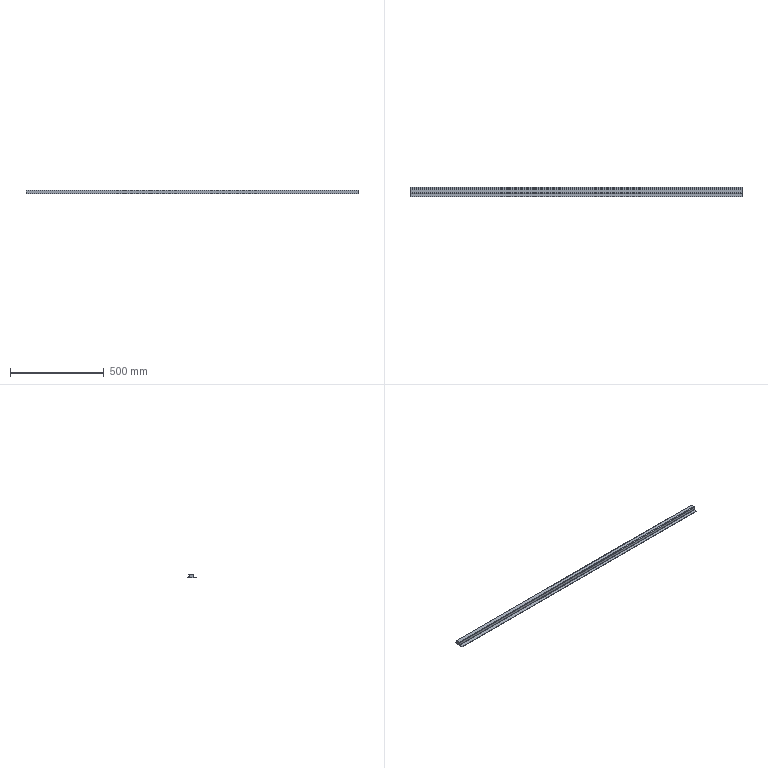Part | SolidWorks | features BaseBody 3 | 3 solids | 54 faces | box 1772 x 51 x 20 mm | volume 297636 mm3 | plane 42 | cylinder 12 | commonest cylinder face diameters 2 x8 6 x4
STEP:
#1=CARTESIAN_POINT('',(-885.9,20.5,-18.));
#2=VERTEX_POINT('',#1);
#3=CARTESIAN_POINT('',(885.9,20.5,-18.));
#4=VERTEX_POINT('',#3);
#5=CARTESIAN_POINT('',(885.9,20.5,-18.));
#6=DIRECTION('',(1.,0.,0.));
#7=VECTOR('',#6,1000.);
#8=LINE('',#5,#7);
#9=EDGE_CURVE('',#2,#4,#8,.T.);
#10=ORIENTED_EDGE('',*,*,#9,.T.);
#11=CARTESIAN_POINT('',(885.9,20.5,-20.));
#12=VERTEX_POINT('',#11);
#13=CARTESIAN_POINT('',(885.9,20.5,-20.));
#14=DIRECTION('',(0.,0.,1.));
#15=VECTOR('',#14,1000.);
#16=LINE('',#13,#15);
#17=EDGE_CURVE('',#12,#4,#16,.T.);
#18=ORIENTED_EDGE('',*,*,#17,.F.);
#19=CARTESIAN_POINT('',(-885.9,20.5,-20.));
#20=VERTEX_POINT('',#19);
#21=CARTESIAN_POINT('',(0.,20.5,-20.));
#22=DIRECTION('',(1.,0.,0.));
#23=VECTOR('',#22,1000.);
#24=LINE('',#21,#23);
#25=EDGE_CURVE('',#20,#12,#24,.T.);
#26=ORIENTED_EDGE('',*,*,#25,.F.);
#27=CARTESIAN_POINT('',(-885.9,20.5,-20.));
#28=DIRECTION('',(0.,0.,1.));
#29=VECTOR('',#28,1000.);
#30=LINE('',#27,#29);
#31=EDGE_CURVE('',#20,#2,#30,.T.);
#32=ORIENTED_EDGE('',*,*,#31,.T.);
#33=EDGE_LOOP('',(#10,#18,#26,#32));
#34=FACE_OUTER_BOUND('',#33,.T.);
#35=CARTESIAN_POINT('',(885.9,20.5,-20.));
#36=DIRECTION('',(0.,-1.,0.));
#37=DIRECTION('',(-1.,0.,0.));
#38=AXIS2_PLACEMENT_3D('',#35,#36,#37);
#39=PLANE('',#38);
#40=ADVANCED_FACE('',(#34),#39,.F.);
#41=CARTESIAN_POINT('',(-885.9,13.5,-18.));
#42=VERTEX_POINT('',#41);
#43=CARTESIAN_POINT('',(-885.9,20.5,-18.));
#44=DIRECTION('',(0.,1.,0.));
#45=VECTOR('',#44,1000.);
#46=LINE('',#43,#45);
#47=EDGE_CURVE('',#42,#2,#46,.T.);
#48=ORIENTED_EDGE('',*,*,#47,.F.);
#49=CARTESIAN_POINT('',(885.9,13.5,-18.));
#50=VERTEX_POINT('',#49);
#51=CARTESIAN_POINT('',(885.9,13.5,-18.));
#52=DIRECTION('',(-1.,0.,0.));
#53=VECTOR('',#52,1000.);
#54=LINE('',#51,#53);
#55=EDGE_CURVE('',#50,#42,#54,.T.);
#56=ORIENTED_EDGE('',*,*,#55,.F.);
#57=CARTESIAN_POINT('',(885.9,12.5,-18.));
#58=DIRECTION('',(0.,-1.,0.));
#59=VECTOR('',#58,1000.);
#60=LINE('',#57,#59);
#61=EDGE_CURVE('',#4,#50,#60,.T.);
#62=ORIENTED_EDGE('',*,*,#61,.F.);
#63=ORIENTED_EDGE('',*,*,#9,.F.);
#64=EDGE_LOOP('',(#48,#56,#62,#63));
#65=FACE_OUTER_BOUND('',#64,.T.);
#66=CARTESIAN_POINT('',(0.,0.,-18.));
#67=DIRECTION('',(0.,0.,1.));
#68=DIRECTION('',(1.,0.,0.));
#69=AXIS2_PLACEMENT_3D('',#66,#67,#68);
#70=PLANE('',#69);
#71=ADVANCED_FACE('',(#65),#70,.T.);
#72=CARTESIAN_POINT('',(-885.9,13.5,-20.));
#73=VERTEX_POINT('',#72);
#74=CARTESIAN_POINT('',(885.9,13.5,-20.));
#75=VERTEX_POINT('',#74);
#76=CARTESIAN_POINT('',(885.9,13.5,-20.));
#77=DIRECTION('',(1.,0.,0.));
#78=VECTOR('',#77,1000.);
#79=LINE('',#76,#78);
#80=EDGE_CURVE('',#73,#75,#79,.T.);
#81=ORIENTED_EDGE('',*,*,#80,.F.);
#82=CARTESIAN_POINT('',(-885.9,0.,-20.));
#83=DIRECTION('',(0.,1.,0.));
#84=VECTOR('',#83,1000.);
#85=LINE('',#82,#84);
#86=EDGE_CURVE('',#73,#20,#85,.T.);
#87=ORIENTED_EDGE('',*,*,#86,.T.);
#88=ORIENTED_EDGE('',*,*,#25,.T.);
#89=CARTESIAN_POINT('',(885.9,0.,-20.));
#90=DIRECTION('',(0.,-1.,0.));
#91=VECTOR('',#90,1000.);
#92=LINE('',#89,#91);
#93=EDGE_CURVE('',#12,#75,#92,.T.);
#94=ORIENTED_EDGE('',*,*,#93,.T.);
#95=EDGE_LOOP('',(#81,#87,#88,#94));
#96=FACE_OUTER_BOUND('',#95,.T.);
#97=CARTESIAN_POINT('',(0.,0.,-20.));
#98=DIRECTION('',(0.,0.,1.));
#99=DIRECTION('',(1.,0.,0.));
#100=AXIS2_PLACEMENT_3D('',#97,#98,#99);
#101=PLANE('',#100);
#102=ADVANCED_FACE('',(#96),#101,.F.);
#103=CARTESIAN_POINT('',(885.9,13.5,-20.));
#104=DIRECTION('',(0.,0.,-1.));
#105=VECTOR('',#104,1000.);
#106=LINE('',#103,#105);
#107=EDGE_CURVE('',#50,#75,#106,.T.);
#108=ORIENTED_EDGE('',*,*,#107,.T.);
#109=ORIENTED_EDGE('',*,*,#93,.F.);
#110=ORIENTED_EDGE('',*,*,#17,.T.);
#111=ORIENTED_EDGE('',*,*,#61,.T.);
#112=EDGE_LOOP('',(#108,#109,#110,#111));
#113=FACE_OUTER_BOUND('',#112,.T.);
#114=CARTESIAN_POINT('',(885.9,12.5,-20.));
#115=DIRECTION('',(-1.,0.,0.));
#116=DIRECTION('',(0.,0.,1.));
#117=AXIS2_PLACEMENT_3D('',#114,#115,#116);
#118=PLANE('',#117);
#119=ADVANCED_FACE('',(#113),#118,.F.);
#120=CARTESIAN_POINT('',(-885.9,13.5,-18.));
#121=DIRECTION('',(0.,0.,-1.));
#122=VECTOR('',#121,1000.);
#123=LINE('',#120,#122);
#124=EDGE_CURVE('',#42,#73,#123,.T.);
#125=ORIENTED_EDGE('',*,*,#124,.F.);
#126=ORIENTED_EDGE('',*,*,#47,.T.);
#127=ORIENTED_EDGE('',*,*,#31,.F.);
#128=ORIENTED_EDGE('',*,*,#86,.F.);
#129=EDGE_LOOP('',(#125,#126,#127,#128));
#130=FACE_OUTER_BOUND('',#129,.T.);
#131=CARTESIAN_POINT('',(-885.9,20.5,-20.));
#132=DIRECTION('',(1.,0.,0.));
#133=DIRECTION('',(0.,1.,0.));
#134=AXIS2_PLACEMENT_3D('',#131,#132,#133);
#135=PLANE('',#134);
#136=ADVANCED_FACE('',(#130),#135,.F.);
#137=CARTESIAN_POINT('',(-885.9,12.5,-17.));
#138=VERTEX_POINT('',#137);
#139=CARTESIAN_POINT('',(885.9,12.5,-17.));
#140=VERTEX_POINT('',#139);
#141=CARTESIAN_POINT('',(-885.9,12.5,-17.));
#142=DIRECTION('',(1.,0.,0.));
#143=VECTOR('',#142,1000.);
#144=LINE('',#141,#143);
#145=EDGE_CURVE('',#138,#140,#144,.T.);
#146=ORIENTED_EDGE('',*,*,#145,.T.);
#147=CARTESIAN_POINT('',(885.9,13.5,-17.));
#148=DIRECTION('',(1.,0.,0.));
#149=DIRECTION('',(0.,0.,1.));
#150=AXIS2_PLACEMENT_3D('',#147,#148,#149);
#151=CIRCLE('',#150,1.);
#152=EDGE_CURVE('',#140,#50,#151,.T.);
#153=ORIENTED_EDGE('',*,*,#152,.T.);
#154=ORIENTED_EDGE('',*,*,#55,.T.);
#155=CARTESIAN_POINT('',(-885.9,13.5,-17.));
#156=DIRECTION('',(-1.,0.,0.));
#157=DIRECTION('',(0.,0.,1.));
#158=AXIS2_PLACEMENT_3D('',#155,#156,#157);
#159=CIRCLE('',#158,1.);
#160=EDGE_CURVE('',#42,#138,#159,.T.);
#161=ORIENTED_EDGE('',*,*,#160,.T.);
#162=EDGE_LOOP('',(#146,#153,#154,#161));
#163=FACE_OUTER_BOUND('',#162,.T.);
#164=CARTESIAN_POINT('',(-885.9,13.5,-17.));
#165=DIRECTION('',(-1.,0.,0.));
#166=DIRECTION('',(0.,0.,-1.));
#167=AXIS2_PLACEMENT_3D('',#164,#165,#166);
#168=CYLINDRICAL_SURFACE('',#167,1.);
#169=ADVANCED_FACE('',(#163),#168,.F.);
#170=CARTESIAN_POINT('',(-885.9,10.5,-17.));
#171=VERTEX_POINT('',#170);
#172=CARTESIAN_POINT('',(885.9,10.5,-17.));
#173=VERTEX_POINT('',#172);
#174=CARTESIAN_POINT('',(-885.9,10.5,-17.));
#175=DIRECTION('',(1.,0.,0.));
#176=VECTOR('',#175,1000.);
#177=LINE('',#174,#176);
#178=EDGE_CURVE('',#171,#173,#177,.T.);
#179=ORIENTED_EDGE('',*,*,#178,.F.);
#180=CARTESIAN_POINT('',(-885.9,13.5,-17.));
#181=DIRECTION('',(-1.,0.,0.));
#182=DIRECTION('',(0.,0.,1.));
#183=AXIS2_PLACEMENT_3D('',#180,#181,#182);
#184=CIRCLE('',#183,3.);
#185=EDGE_CURVE('',#73,#171,#184,.T.);
#186=ORIENTED_EDGE('',*,*,#185,.F.);
#187=ORIENTED_EDGE('',*,*,#80,.T.);
#188=CARTESIAN_POINT('',(885.9,13.5,-17.));
#189=DIRECTION('',(1.,0.,0.));
#190=DIRECTION('',(0.,0.,1.));
#191=AXIS2_PLACEMENT_3D('',#188,#189,#190);
#192=CIRCLE('',#191,3.);
#193=EDGE_CURVE('',#173,#75,#192,.T.);
#194=ORIENTED_EDGE('',*,*,#193,.F.);
#195=EDGE_LOOP('',(#179,#186,#187,#194));
#196=FACE_OUTER_BOUND('',#195,.T.);
#197=CARTESIAN_POINT('',(-885.9,13.5,-17.));
#198=DIRECTION('',(-1.,0.,0.));
#199=DIRECTION('',(0.,0.,-1.));
#200=AXIS2_PLACEMENT_3D('',#197,#198,#199);
#201=CYLINDRICAL_SURFACE('',#200,3.);
#202=ADVANCED_FACE('',(#196),#201,.T.);
#203=ORIENTED_EDGE('',*,*,#160,.F.);
#204=ORIENTED_EDGE('',*,*,#124,.T.);
#205=ORIENTED_EDGE('',*,*,#185,.T.);
#206=CARTESIAN_POINT('',(-885.9,12.5,-17.));
#207=DIRECTION('',(0.,-1.,0.));
#208=VECTOR('',#207,1000.);
#209=LINE('',#206,#208);
#210=EDGE_CURVE('',#138,#171,#209,.T.);
#211=ORIENTED_EDGE('',*,*,#210,.F.);
#212=EDGE_LOOP('',(#203,#204,#205,#211));
#213=FACE_OUTER_BOUND('',#212,.T.);
#214=CARTESIAN_POINT('',(-885.9,13.5,-17.));
#215=DIRECTION('',(1.,0.,0.));
#216=DIRECTION('',(0.,1.,0.));
#217=AXIS2_PLACEMENT_3D('',#214,#215,#216);
#218=PLANE('',#217);
#219=ADVANCED_FACE('',(#213),#218,.F.);
#220=ORIENTED_EDGE('',*,*,#107,.F.);
#221=ORIENTED_EDGE('',*,*,#152,.F.);
#222=CARTESIAN_POINT('',(885.9,12.5,-17.));
#223=DIRECTION('',(0.,-1.,0.));
#224=VECTOR('',#223,1000.);
#225=LINE('',#222,#224);
#226=EDGE_CURVE('',#140,#173,#225,.T.);
#227=ORIENTED_EDGE('',*,*,#226,.T.);
#228=ORIENTED_EDGE('',*,*,#193,.T.);
#229=EDGE_LOOP('',(#220,#221,#227,#228));
#230=FACE_OUTER_BOUND('',#229,.T.);
#231=CARTESIAN_POINT('',(885.9,13.5,-17.));
#232=DIRECTION('',(1.,0.,0.));
#233=DIRECTION('',(0.,1.,0.));
#234=AXIS2_PLACEMENT_3D('',#231,#232,#233);
#235=PLANE('',#234);
#236=ADVANCED_FACE('',(#230),#235,.T.);
#237=CARTESIAN_POINT('',(-885.9,-30.5,-18.));
#238=VERTEX_POINT('',#237);
#239=CARTESIAN_POINT('',(885.9,-30.5,-18.));
#240=VERTEX_POINT('',#239);
#241=CARTESIAN_POINT('',(0.,-30.5,-18.));
#242=DIRECTION('',(1.,0.,0.));
#243=VECTOR('',#242,1000.);
#244=LINE('',#241,#243);
#245=EDGE_CURVE('',#238,#240,#244,.T.);
#246=ORIENTED_EDGE('',*,*,#245,.F.);
#247=CARTESIAN_POINT('',(-885.9,-30.5,-20.));
#248=VERTEX_POINT('',#247);
#249=CARTESIAN_POINT('',(-885.9,-30.5,-20.));
#250=DIRECTION('',(0.,0.,1.));
#251=VECTOR('',#250,1000.);
#252=LINE('',#249,#251);
#253=EDGE_CURVE('',#248,#238,#252,.T.);
#254=ORIENTED_EDGE('',*,*,#253,.F.);
#255=CARTESIAN_POINT('',(885.9,-30.5,-20.));
#256=VERTEX_POINT('',#255);
#257=CARTESIAN_POINT('',(-885.9,-30.5,-20.));
#258=DIRECTION('',(1.,0.,0.));
#259=VECTOR('',#258,1000.);
#260=LINE('',#257,#259);
#261=EDGE_CURVE('',#248,#256,#260,.T.);
#262=ORIENTED_EDGE('',*,*,#261,.T.);
#263=CARTESIAN_POINT('',(885.9,-30.5,-20.));
#264=DIRECTION('',(0.,0.,1.));
#265=VECTOR('',#264,1000.);
#266=LINE('',#263,#265);
#267=EDGE_CURVE('',#256,#240,#266,.T.);
#268=ORIENTED_EDGE('',*,*,#267,.T.);
#269=EDGE_LOOP('',(#246,#254,#262,#268));
#270=FACE_OUTER_BOUND('',#269,.T.);
#271=CARTESIAN_POINT('',(-885.9,-30.5,-20.));
#272=DIRECTION('',(0.,-1.,0.));
#273=DIRECTION('',(0.,0.,-1.));
#274=AXIS2_PLACEMENT_3D('',#271,#272,#273);
#275=PLANE('',#274);
#276=ADVANCED_FACE('',(#270),#275,.T.);
#277=CARTESIAN_POINT('',(885.9,-13.5,-18.));
#278=VERTEX_POINT('',#277);
#279=CARTESIAN_POINT('',(885.9,0.,-18.));
#280=DIRECTION('',(0.,1.,0.));
#281=VECTOR('',#280,1000.);
#282=LINE('',#279,#281);
#283=EDGE_CURVE('',#240,#278,#282,.T.);
#284=ORIENTED_EDGE('',*,*,#283,.T.);
#285=CARTESIAN_POINT('',(-885.9,-13.5,-18.));
#286=VERTEX_POINT('',#285);
#287=CARTESIAN_POINT('',(-885.9,-13.5,-18.));
#288=DIRECTION('',(1.,0.,0.));
#289=VECTOR('',#288,1000.);
#290=LINE('',#287,#289);
#291=EDGE_CURVE('',#286,#278,#290,.T.);
#292=ORIENTED_EDGE('',*,*,#291,.F.);
#293=CARTESIAN_POINT('',(-885.9,0.,-18.));
#294=DIRECTION('',(0.,-1.,0.));
#295=VECTOR('',#294,1000.);
#296=LINE('',#293,#295);
#297=EDGE_CURVE('',#286,#238,#296,.T.);
#298=ORIENTED_EDGE('',*,*,#297,.T.);
#299=ORIENTED_EDGE('',*,*,#245,.T.);
#300=EDGE_LOOP('',(#284,#292,#298,#299));
#301=FACE_OUTER_BOUND('',#300,.T.);
#302=CARTESIAN_POINT('',(0.,0.,-18.));
#303=DIRECTION('',(0.,0.,1.));
#304=DIRECTION('',(1.,0.,0.));
#305=AXIS2_PLACEMENT_3D('',#302,#303,#304);
#306=PLANE('',#305);
#307=ADVANCED_FACE('',(#301),#306,.T.);
#308=CARTESIAN_POINT('',(885.9,-13.5,-20.));
#309=VERTEX_POINT('',#308);
#310=CARTESIAN_POINT('',(-885.9,-13.5,-20.));
#311=VERTEX_POINT('',#310);
#312=CARTESIAN_POINT('',(-885.9,-13.5,-20.));
#313=DIRECTION('',(-1.,0.,0.));
#314=VECTOR('',#313,1000.);
#315=LINE('',#312,#314);
#316=EDGE_CURVE('',#309,#311,#315,.T.);
#317=ORIENTED_EDGE('',*,*,#316,.F.);
#318=CARTESIAN_POINT('',(885.9,-30.5,-20.));
#319=DIRECTION('',(0.,1.,0.));
#320=VECTOR('',#319,1000.);
#321=LINE('',#318,#320);
#322=EDGE_CURVE('',#256,#309,#321,.T.);
#323=ORIENTED_EDGE('',*,*,#322,.F.);
#324=ORIENTED_EDGE('',*,*,#261,.F.);
#325=CARTESIAN_POINT('',(-885.9,-12.5,-20.));
#326=DIRECTION('',(0.,-1.,0.));
#327=VECTOR('',#326,1000.);
#328=LINE('',#325,#327);
#329=EDGE_CURVE('',#311,#248,#328,.T.);
#330=ORIENTED_EDGE('',*,*,#329,.F.);
#331=EDGE_LOOP('',(#317,#323,#324,#330));
#332=FACE_OUTER_BOUND('',#331,.T.);
#333=CARTESIAN_POINT('',(0.,0.,-20.));
#334=DIRECTION('',(0.,0.,1.));
#335=DIRECTION('',(1.,0.,0.));
#336=AXIS2_PLACEMENT_3D('',#333,#334,#335);
#337=PLANE('',#336);
#338=ADVANCED_FACE('',(#332),#337,.F.);
#339=ORIENTED_EDGE('',*,*,#322,.T.);
#340=CARTESIAN_POINT('',(885.9,-13.5,-18.));
#341=DIRECTION('',(0.,0.,-1.));
#342=VECTOR('',#341,1000.);
#343=LINE('',#340,#342);
#344=EDGE_CURVE('',#278,#309,#343,.T.);
#345=ORIENTED_EDGE('',*,*,#344,.F.);
#346=ORIENTED_EDGE('',*,*,#283,.F.);
#347=ORIENTED_EDGE('',*,*,#267,.F.);
#348=EDGE_LOOP('',(#339,#345,#346,#347));
#349=FACE_OUTER_BOUND('',#348,.T.);
#350=CARTESIAN_POINT('',(885.9,-30.5,-20.));
#351=DIRECTION('',(1.,0.,0.));
#352=DIRECTION('',(0.,0.,-1.));
#353=AXIS2_PLACEMENT_3D('',#350,#351,#352);
#354=PLANE('',#353);
#355=ADVANCED_FACE('',(#349),#354,.T.);
#356=ORIENTED_EDGE('',*,*,#297,.F.);
#357=CARTESIAN_POINT('',(-885.9,-13.5,-20.));
#358=DIRECTION('',(0.,0.,-1.));
#359=VECTOR('',#358,1000.);
#360=LINE('',#357,#359);
#361=EDGE_CURVE('',#286,#311,#360,.T.);
#362=ORIENTED_EDGE('',*,*,#361,.T.);
#363=ORIENTED_EDGE('',*,*,#329,.T.);
#364=ORIENTED_EDGE('',*,*,#253,.T.);
#365=EDGE_LOOP('',(#356,#362,#363,#364));
#366=FACE_OUTER_BOUND('',#365,.T.);
#367=CARTESIAN_POINT('',(-885.9,-12.5,-20.));
#368=DIRECTION('',(-1.,0.,0.));
#369=DIRECTION('',(0.,1.,0.));
#370=AXIS2_PLACEMENT_3D('',#367,#368,#369);
#371=PLANE('',#370);
#372=ADVANCED_FACE('',(#366),#371,.T.);
#373=CARTESIAN_POINT('',(885.9,-12.5,-17.));
#374=VERTEX_POINT('',#373);
#375=CARTESIAN_POINT('',(-885.9,-12.5,-17.));
#376=VERTEX_POINT('',#375);
#377=CARTESIAN_POINT('',(885.9,-12.5,-17.));
#378=DIRECTION('',(-1.,0.,0.));
#379=VECTOR('',#378,1000.);
#380=LINE('',#377,#379);
#381=EDGE_CURVE('',#374,#376,#380,.T.);
#382=ORIENTED_EDGE('',*,*,#381,.T.);
#383=CARTESIAN_POINT('',(-885.9,-13.5,-17.));
#384=DIRECTION('',(-1.,0.,0.));
#385=DIRECTION('',(0.,0.,-1.));
#386=AXIS2_PLACEMENT_3D('',#383,#384,#385);
#387=CIRCLE('',#386,1.);
#388=EDGE_CURVE('',#376,#286,#387,.T.);
#389=ORIENTED_EDGE('',*,*,#388,.T.);
#390=ORIENTED_EDGE('',*,*,#291,.T.);
#391=CARTESIAN_POINT('',(885.9,-13.5,-17.));
#392=DIRECTION('',(1.,0.,0.));
#393=DIRECTION('',(0.,0.,-1.));
#394=AXIS2_PLACEMENT_3D('',#391,#392,#393);
#395=CIRCLE('',#394,1.);
#396=EDGE_CURVE('',#278,#374,#395,.T.);
#397=ORIENTED_EDGE('',*,*,#396,.T.);
#398=EDGE_LOOP('',(#382,#389,#390,#397));
#399=FACE_OUTER_BOUND('',#398,.T.);
#400=CARTESIAN_POINT('',(885.9,-13.5,-17.));
#401=DIRECTION('',(1.,0.,0.));
#402=DIRECTION('',(0.,0.,-1.));
#403=AXIS2_PLACEMENT_3D('',#400,#401,#402);
#404=CYLINDRICAL_SURFACE('',#403,1.);
#405=ADVANCED_FACE('',(#399),#404,.F.);
#406=CARTESIAN_POINT('',(885.9,-10.5,-17.));
#407=VERTEX_POINT('',#406);
#408=CARTESIAN_POINT('',(-885.9,-10.5,-17.));
#409=VERTEX_POINT('',#408);
#410=CARTESIAN_POINT('',(885.9,-10.5,-17.));
#411=DIRECTION('',(-1.,0.,0.));
#412=VECTOR('',#411,1000.);
#413=LINE('',#410,#412);
#414=EDGE_CURVE('',#407,#409,#413,.T.);
#415=ORIENTED_EDGE('',*,*,#414,.F.);
#416=CARTESIAN_POINT('',(885.9,-13.5,-17.));
#417=DIRECTION('',(1.,0.,0.));
#418=DIRECTION('',(0.,0.,-1.));
#419=AXIS2_PLACEMENT_3D('',#416,#417,#418);
#420=CIRCLE('',#419,3.);
#421=EDGE_CURVE('',#309,#407,#420,.T.);
#422=ORIENTED_EDGE('',*,*,#421,.F.);
#423=ORIENTED_EDGE('',*,*,#316,.T.);
#424=CARTESIAN_POINT('',(-885.9,-13.5,-17.));
#425=DIRECTION('',(-1.,0.,0.));
#426=DIRECTION('',(0.,0.,-1.));
#427=AXIS2_PLACEMENT_3D('',#424,#425,#426);
#428=CIRCLE('',#427,3.);
#429=EDGE_CURVE('',#409,#311,#428,.T.);
#430=ORIENTED_EDGE('',*,*,#429,.F.);
#431=EDGE_LOOP('',(#415,#422,#423,#430));
#432=FACE_OUTER_BOUND('',#431,.T.);
#433=CARTESIAN_POINT('',(885.9,-13.5,-17.));
#434=DIRECTION('',(1.,0.,0.));
#435=DIRECTION('',(0.,0.,-1.));
#436=AXIS2_PLACEMENT_3D('',#433,#434,#435);
#437=CYLINDRICAL_SURFACE('',#436,3.);
#438=ADVANCED_FACE('',(#432),#437,.T.);
#439=ORIENTED_EDGE('',*,*,#396,.F.);
#440=ORIENTED_EDGE('',*,*,#344,.T.);
#441=ORIENTED_EDGE('',*,*,#421,.T.);
#442=CARTESIAN_POINT('',(885.9,-12.5,-17.));
#443=DIRECTION('',(0.,1.,0.));
#444=VECTOR('',#443,1000.);
#445=LINE('',#442,#444);
#446=EDGE_CURVE('',#374,#407,#445,.T.);
#447=ORIENTED_EDGE('',*,*,#446,.F.);
#448=EDGE_LOOP('',(#439,#440,#441,#447));
#449=FACE_OUTER_BOUND('',#448,.T.);
#450=CARTESIAN_POINT('',(885.9,-13.5,-17.));
#451=DIRECTION('',(-1.,0.,0.));
#452=DIRECTION('',(0.,0.,1.));
#453=AXIS2_PLACEMENT_3D('',#450,#451,#452);
#454=PLANE('',#453);
#455=ADVANCED_FACE('',(#449),#454,.F.);
#456=ORIENTED_EDGE('',*,*,#361,.F.);
#457=ORIENTED_EDGE('',*,*,#388,.F.);
#458=CARTESIAN_POINT('',(-885.9,-12.5,-17.));
#459=DIRECTION('',(0.,1.,0.));
#460=VECTOR('',#459,1000.);
#461=LINE('',#458,#460);
#462=EDGE_CURVE('',#376,#409,#461,.T.);
#463=ORIENTED_EDGE('',*,*,#462,.T.);
#464=ORIENTED_EDGE('',*,*,#429,.T.);
#465=EDGE_LOOP('',(#456,#457,#463,#464));
#466=FACE_OUTER_BOUND('',#465,.T.);
#467=CARTESIAN_POINT('',(-885.9,-13.5,-17.));
#468=DIRECTION('',(-1.,0.,0.));
#469=DIRECTION('',(0.,0.,1.));
#470=AXIS2_PLACEMENT_3D('',#467,#468,#469);
#471=PLANE('',#470);
#472=ADVANCED_FACE('',(#466),#471,.T.);
#473=ORIENTED_EDGE('',*,*,#462,.F.);
#474=CARTESIAN_POINT('',(-885.9,-12.5,-3.));
#475=VERTEX_POINT('',#474);
#476=CARTESIAN_POINT('',(-885.9,-12.5,-20.));
#477=DIRECTION('',(0.,0.,1.));
#478=VECTOR('',#477,1000.);
#479=LINE('',#476,#478);
#480=EDGE_CURVE('',#376,#475,#479,.T.);
#481=ORIENTED_EDGE('',*,*,#480,.T.);
#482=CARTESIAN_POINT('',(-885.9,-10.5,-3.));
#483=VERTEX_POINT('',#482);
#484=CARTESIAN_POINT('',(-885.9,-10.5,-3.));
#485=DIRECTION('',(0.,-1.,0.));
#486=VECTOR('',#485,1000.);
#487=LINE('',#484,#486);
#488=EDGE_CURVE('',#483,#475,#487,.T.);
#489=ORIENTED_EDGE('',*,*,#488,.F.);
#490=CARTESIAN_POINT('',(-885.9,-10.5,0.));
#491=DIRECTION('',(0.,0.,1.));
#492=VECTOR('',#491,1000.);
#493=LINE('',#490,#492);
#494=EDGE_CURVE('',#409,#483,#493,.T.);
#495=ORIENTED_EDGE('',*,*,#494,.F.);
#496=EDGE_LOOP('',(#473,#481,#489,#495));
#497=FACE_OUTER_BOUND('',#496,.T.);
#498=CARTESIAN_POINT('',(-885.9,-12.5,-20.));
#499=DIRECTION('',(-1.,0.,0.));
#500=DIRECTION('',(0.,0.,1.));
#501=AXIS2_PLACEMENT_3D('',#498,#499,#500);
#502=PLANE('',#501);
#503=ADVANCED_FACE('',(#497),#502,.T.);
#504=CARTESIAN_POINT('',(-885.9,-9.5,-2.));
#505=VERTEX_POINT('',#504);
#506=CARTESIAN_POINT('',(885.9,-9.5,-2.));
#507=VERTEX_POINT('',#506);
#508=CARTESIAN_POINT('',(-885.9,-9.5,-2.));
#509=DIRECTION('',(1.,0.,0.));
#510=VECTOR('',#509,1000.);
#511=LINE('',#508,#510);
#512=EDGE_CURVE('',#505,#507,#511,.T.);
#513=ORIENTED_EDGE('',*,*,#512,.T.);
#514=CARTESIAN_POINT('',(885.9,-10.5,-3.));
#515=VERTEX_POINT('',#514);
#516=CARTESIAN_POINT('',(885.9,-9.5,-3.));
#517=DIRECTION('',(1.,0.,0.));
#518=DIRECTION('',(0.,0.,1.));
#519=AXIS2_PLACEMENT_3D('',#516,#517,#518);
#520=CIRCLE('',#519,1.);
#521=EDGE_CURVE('',#507,#515,#520,.T.);
#522=ORIENTED_EDGE('',*,*,#521,.T.);
#523=CARTESIAN_POINT('',(885.9,-10.5,-3.));
#524=DIRECTION('',(-1.,0.,0.));
#525=VECTOR('',#524,1000.);
#526=LINE('',#523,#525);
#527=EDGE_CURVE('',#515,#483,#526,.T.);
#528=ORIENTED_EDGE('',*,*,#527,.T.);
#529=CARTESIAN_POINT('',(-885.9,-9.5,-3.));
#530=DIRECTION('',(-1.,0.,0.));
#531=DIRECTION('',(0.,0.,1.));
#532=AXIS2_PLACEMENT_3D('',#529,#530,#531);
#533=CIRCLE('',#532,1.);
#534=EDGE_CURVE('',#483,#505,#533,.T.);
#535=ORIENTED_EDGE('',*,*,#534,.T.);
#536=EDGE_LOOP('',(#513,#522,#528,#535));
#537=FACE_OUTER_BOUND('',#536,.T.);
#538=CARTESIAN_POINT('',(-885.9,-9.5,-3.));
#539=DIRECTION('',(-1.,0.,0.));
#540=DIRECTION('',(0.,-1.,0.));
#541=AXIS2_PLACEMENT_3D('',#538,#539,#540);
#542=CYLINDRICAL_SURFACE('',#541,1.);
#543=ADVANCED_FACE('',(#537),#542,.F.);
#544=CARTESIAN_POINT('',(-885.9,-9.5,0.));
#545=VERTEX_POINT('',#544);
#546=CARTESIAN_POINT('',(885.9,-9.5,0.));
#547=VERTEX_POINT('',#546);
#548=CARTESIAN_POINT('',(-885.9,-9.5,0.));
#549=DIRECTION('',(1.,0.,0.));
#550=VECTOR('',#549,1000.);
#551=LINE('',#548,#550);
#552=EDGE_CURVE('',#545,#547,#551,.T.);
#553=ORIENTED_EDGE('',*,*,#552,.F.);
#554=CARTESIAN_POINT('',(-885.9,-9.5,-3.));
#555=DIRECTION('',(-1.,0.,0.));
#556=DIRECTION('',(0.,0.,1.));
#557=AXIS2_PLACEMENT_3D('',#554,#555,#556);
#558=CIRCLE('',#557,3.);
#559=EDGE_CURVE('',#475,#545,#558,.T.);
#560=ORIENTED_EDGE('',*,*,#559,.F.);
#561=CARTESIAN_POINT('',(885.9,-12.5,-3.));
#562=VERTEX_POINT('',#561);
#563=CARTESIAN_POINT('',(885.9,-12.5,-3.));
#564=DIRECTION('',(1.,0.,0.));
#565=VECTOR('',#564,1000.);
#566=LINE('',#563,#565);
#567=EDGE_CURVE('',#475,#562,#566,.T.);
#568=ORIENTED_EDGE('',*,*,#567,.T.);
#569=CARTESIAN_POINT('',(885.9,-9.5,-3.));
#570=DIRECTION('',(1.,0.,0.));
#571=DIRECTION('',(0.,0.,1.));
#572=AXIS2_PLACEMENT_3D('',#569,#570,#571);
#573=CIRCLE('',#572,3.);
#574=EDGE_CURVE('',#547,#562,#573,.T.);
#575=ORIENTED_EDGE('',*,*,#574,.F.);
#576=EDGE_LOOP('',(#553,#560,#568,#575));
#577=FACE_OUTER_BOUND('',#576,.T.);
#578=CARTESIAN_POINT('',(-885.9,-9.5,-3.));
#579=DIRECTION('',(-1.,0.,0.));
#580=DIRECTION('',(0.,-1.,0.));
#581=AXIS2_PLACEMENT_3D('',#578,#579,#580);
#582=CYLINDRICAL_SURFACE('',#581,3.);
#583=ADVANCED_FACE('',(#577),#582,.T.);
#584=ORIENTED_EDGE('',*,*,#534,.F.);
#585=ORIENTED_EDGE('',*,*,#488,.T.);
#586=ORIENTED_EDGE('',*,*,#559,.T.);
#587=CARTESIAN_POINT('',(-885.9,-9.5,-2.));
#588=DIRECTION('',(0.,0.,1.));
#589=VECTOR('',#588,1000.);
#590=LINE('',#587,#589);
#591=EDGE_CURVE('',#505,#545,#590,.T.);
#592=ORIENTED_EDGE('',*,*,#591,.F.);
#593=EDGE_LOOP('',(#584,#585,#586,#592));
#594=FACE_OUTER_BOUND('',#593,.T.);
#595=CARTESIAN_POINT('',(-885.9,-9.5,-3.));
#596=DIRECTION('',(1.,0.,0.));
#597=DIRECTION('',(0.,1.,0.));
#598=AXIS2_PLACEMENT_3D('',#595,#596,#597);
#599=PLANE('',#598);
#600=ADVANCED_FACE('',(#594),#599,.F.);
#601=CARTESIAN_POINT('',(885.9,-12.5,-3.));
#602=DIRECTION('',(0.,-1.,0.));
#603=VECTOR('',#602,1000.);
#604=LINE('',#601,#603);
#605=EDGE_CURVE('',#515,#562,#604,.T.);
#606=ORIENTED_EDGE('',*,*,#605,.F.);
#607=ORIENTED_EDGE('',*,*,#521,.F.);
#608=CARTESIAN_POINT('',(885.9,-9.5,-2.));
#609=DIRECTION('',(0.,0.,1.));
#610=VECTOR('',#609,1000.);
#611=LINE('',#608,#610);
#612=EDGE_CURVE('',#507,#547,#611,.T.);
#613=ORIENTED_EDGE('',*,*,#612,.T.);
#614=ORIENTED_EDGE('',*,*,#574,.T.);
#615=EDGE_LOOP('',(#606,#607,#613,#614));
#616=FACE_OUTER_BOUND('',#615,.T.);
#617=CARTESIAN_POINT('',(885.9,-9.5,-3.));
#618=DIRECTION('',(1.,0.,0.));
#619=DIRECTION('',(0.,1.,0.));
#620=AXIS2_PLACEMENT_3D('',#617,#618,#619);
#621=PLANE('',#620);
#622=ADVANCED_FACE('',(#616),#621,.T.);
#623=ORIENTED_EDGE('',*,*,#226,.F.);
#624=CARTESIAN_POINT('',(885.9,12.5,-3.));
#625=VERTEX_POINT('',#624);
#626=CARTESIAN_POINT('',(885.9,12.5,-2.));
#627=DIRECTION('',(0.,0.,1.));
#628=VECTOR('',#627,1000.);
#629=LINE('',#626,#628);
#630=EDGE_CURVE('',#140,#625,#629,.T.);
#631=ORIENTED_EDGE('',*,*,#630,.T.);
#632=CARTESIAN_POINT('',(885.9,10.5,-3.));
#633=VERTEX_POINT('',#632);
#634=CARTESIAN_POINT('',(885.9,10.5,-3.));
#635=DIRECTION('',(0.,1.,0.));
#636=VECTOR('',#635,1000.);
#637=LINE('',#634,#636);
#638=EDGE_CURVE('',#633,#625,#637,.T.);
#639=ORIENTED_EDGE('',*,*,#638,.F.);
#640=CARTESIAN_POINT('',(885.9,10.5,0.));
#641=DIRECTION('',(0.,0.,1.));
#642=VECTOR('',#641,1000.);
#643=LINE('',#640,#642);
#644=EDGE_CURVE('',#173,#633,#643,.T.);
#645=ORIENTED_EDGE('',*,*,#644,.F.);
#646=EDGE_LOOP('',(#623,#631,#639,#645));
#647=FACE_OUTER_BOUND('',#646,.T.);
#648=CARTESIAN_POINT('',(885.9,12.5,-2.));
#649=DIRECTION('',(1.,0.,0.));
#650=DIRECTION('',(0.,1.,0.));
#651=AXIS2_PLACEMENT_3D('',#648,#649,#650);
#652=PLANE('',#651);
#653=ADVANCED_FACE('',(#647),#652,.T.);
#654=CARTESIAN_POINT('',(885.9,9.5,-2.));
#655=VERTEX_POINT('',#654);
#656=CARTESIAN_POINT('',(-885.9,9.5,-2.));
#657=VERTEX_POINT('',#656);
#658=CARTESIAN_POINT('',(885.9,9.5,-2.));
#659=DIRECTION('',(-1.,0.,0.));
#660=VECTOR('',#659,1000.);
#661=LINE('',#658,#660);
#662=EDGE_CURVE('',#655,#657,#661,.T.);
#663=ORIENTED_EDGE('',*,*,#662,.T.);
#664=CARTESIAN_POINT('',(-885.9,10.5,-3.));
#665=VERTEX_POINT('',#664);
#666=CARTESIAN_POINT('',(-885.9,9.5,-3.));
#667=DIRECTION('',(-1.,0.,0.));
#668=DIRECTION('',(0.,0.,-1.));
#669=AXIS2_PLACEMENT_3D('',#666,#667,#668);
#670=CIRCLE('',#669,1.);
#671=EDGE_CURVE('',#657,#665,#670,.T.);
#672=ORIENTED_EDGE('',*,*,#671,.T.);
#673=CARTESIAN_POINT('',(-885.9,10.5,-3.));
#674=DIRECTION('',(1.,0.,0.));
#675=VECTOR('',#674,1000.);
#676=LINE('',#673,#675);
#677=EDGE_CURVE('',#665,#633,#676,.T.);
#678=ORIENTED_EDGE('',*,*,#677,.T.);
#679=CARTESIAN_POINT('',(885.9,9.5,-3.));
#680=DIRECTION('',(1.,0.,0.));
#681=DIRECTION('',(0.,0.,-1.));
#682=AXIS2_PLACEMENT_3D('',#679,#680,#681);
#683=CIRCLE('',#682,1.);
#684=EDGE_CURVE('',#633,#655,#683,.T.);
#685=ORIENTED_EDGE('',*,*,#684,.T.);
#686=EDGE_LOOP('',(#663,#672,#678,#685));
#687=FACE_OUTER_BOUND('',#686,.T.);
#688=CARTESIAN_POINT('',(885.9,9.5,-3.));
#689=DIRECTION('',(1.,0.,0.));
#690=DIRECTION('',(0.,1.,0.));
#691=AXIS2_PLACEMENT_3D('',#688,#689,#690);
#692=CYLINDRICAL_SURFACE('',#691,1.);
#693=ADVANCED_FACE('',(#687),#692,.F.);
#694=CARTESIAN_POINT('',(885.9,9.5,0.));
#695=VERTEX_POINT('',#694);
#696=CARTESIAN_POINT('',(-885.9,9.5,0.));
#697=VERTEX_POINT('',#696);
#698=CARTESIAN_POINT('',(885.9,9.5,0.));
#699=DIRECTION('',(-1.,0.,0.));
#700=VECTOR('',#699,1000.);
#701=LINE('',#698,#700);
#702=EDGE_CURVE('',#695,#697,#701,.T.);
#703=ORIENTED_EDGE('',*,*,#702,.F.);
#704=CARTESIAN_POINT('',(885.9,9.5,-3.));
#705=DIRECTION('',(1.,0.,0.));
#706=DIRECTION('',(0.,0.,-1.));
#707=AXIS2_PLACEMENT_3D('',#704,#705,#706);
#708=CIRCLE('',#707,3.);
#709=EDGE_CURVE('',#625,#695,#708,.T.);
#710=ORIENTED_EDGE('',*,*,#709,.F.);
#711=CARTESIAN_POINT('',(-885.9,12.5,-3.));
#712=VERTEX_POINT('',#711);
#713=CARTESIAN_POINT('',(0.,12.5,-3.));
#714=DIRECTION('',(1.,0.,0.));
#715=VECTOR('',#714,1000.);
#716=LINE('',#713,#715);
#717=EDGE_CURVE('',#712,#625,#716,.T.);
#718=ORIENTED_EDGE('',*,*,#717,.F.);
#719=CARTESIAN_POINT('',(-885.9,9.5,-3.));
#720=DIRECTION('',(-1.,0.,0.));
#721=DIRECTION('',(0.,0.,-1.));
#722=AXIS2_PLACEMENT_3D('',#719,#720,#721);
#723=CIRCLE('',#722,3.);
#724=EDGE_CURVE('',#697,#712,#723,.T.);
#725=ORIENTED_EDGE('',*,*,#724,.F.);
#726=EDGE_LOOP('',(#703,#710,#718,#725));
#727=FACE_OUTER_BOUND('',#726,.T.);
#728=CARTESIAN_POINT('',(885.9,9.5,-3.));
#729=DIRECTION('',(1.,0.,0.));
#730=DIRECTION('',(0.,1.,0.));
#731=AXIS2_PLACEMENT_3D('',#728,#729,#730);
#732=CYLINDRICAL_SURFACE('',#731,3.);
#733=ADVANCED_FACE('',(#727),#732,.T.);
#734=ORIENTED_EDGE('',*,*,#684,.F.);
#735=ORIENTED_EDGE('',*,*,#638,.T.);
#736=ORIENTED_EDGE('',*,*,#709,.T.);
#737=CARTESIAN_POINT('',(885.9,9.5,-2.));
#738=DIRECTION('',(0.,0.,1.));
#739=VECTOR('',#738,1000.);
#740=LINE('',#737,#739);
#741=EDGE_CURVE('',#655,#695,#740,.T.);
#742=ORIENTED_EDGE('',*,*,#741,.F.);
#743=EDGE_LOOP('',(#734,#735,#736,#742));
#744=FACE_OUTER_BOUND('',#743,.T.);
#745=CARTESIAN_POINT('',(885.9,9.5,-3.));
#746=DIRECTION('',(-1.,0.,0.));
#747=DIRECTION('',(0.,0.,1.));
#748=AXIS2_PLACEMENT_3D('',#745,#746,#747);
#749=PLANE('',#748);
#750=ADVANCED_FACE('',(#744),#749,.F.);
#751=CARTESIAN_POINT('',(-885.9,12.5,-3.));
#752=DIRECTION('',(0.,1.,0.));
#753=VECTOR('',#752,1000.);
#754=LINE('',#751,#753);
#755=EDGE_CURVE('',#665,#712,#754,.T.);
#756=ORIENTED_EDGE('',*,*,#755,.F.);
#757=ORIENTED_EDGE('',*,*,#671,.F.);
#758=CARTESIAN_POINT('',(-885.9,9.5,-2.));
#759=DIRECTION('',(0.,0.,1.));
#760=VECTOR('',#759,1000.);
#761=LINE('',#758,#760);
#762=EDGE_CURVE('',#657,#697,#761,.T.);
#763=ORIENTED_EDGE('',*,*,#762,.T.);
#764=ORIENTED_EDGE('',*,*,#724,.T.);
#765=EDGE_LOOP('',(#756,#757,#763,#764));
#766=FACE_OUTER_BOUND('',#765,.T.);
#767=CARTESIAN_POINT('',(-885.9,9.5,-3.));
#768=DIRECTION('',(-1.,0.,0.));
#769=DIRECTION('',(0.,0.,1.));
#770=AXIS2_PLACEMENT_3D('',#767,#768,#769);
#771=PLANE('',#770);
#772=ADVANCED_FACE('',(#766),#771,.T.);
#773=ORIENTED_EDGE('',*,*,#612,.F.);
#774=CARTESIAN_POINT('',(885.9,12.5,-2.));
#775=DIRECTION('',(0.,1.,0.));
#776=VECTOR('',#775,1000.);
#777=LINE('',#774,#776);
#778=EDGE_CURVE('',#507,#655,#777,.T.);
#779=ORIENTED_EDGE('',*,*,#778,.T.);
#780=ORIENTED_EDGE('',*,*,#741,.T.);
#781=CARTESIAN_POINT('',(885.9,12.5,0.));
#782=DIRECTION('',(0.,1.,0.));
#783=VECTOR('',#782,1000.);
#784=LINE('',#781,#783);
#785=EDGE_CURVE('',#547,#695,#784,.T.);
#786=ORIENTED_EDGE('',*,*,#785,.F.);
#787=EDGE_LOOP('',(#773,#779,#780,#786));
#788=FACE_OUTER_BOUND('',#787,.T.);
#789=CARTESIAN_POINT('',(885.9,12.5,-2.));
#790=DIRECTION('',(1.,0.,0.));
#791=DIRECTION('',(0.,1.,0.));
#792=AXIS2_PLACEMENT_3D('',#789,#790,#791);
#793=PLANE('',#792);
#794=ADVANCED_FACE('',(#788),#793,.T.);
#795=CARTESIAN_POINT('',(-885.9,12.5,-2.));
#796=DIRECTION('',(0.,-1.,0.));
#797=VECTOR('',#796,1000.);
#798=LINE('',#795,#797);
#799=EDGE_CURVE('',#657,#505,#798,.T.);
#800=ORIENTED_EDGE('',*,*,#799,.T.);
#801=ORIENTED_EDGE('',*,*,#591,.T.);
#802=CARTESIAN_POINT('',(-885.9,12.5,0.));
#803=DIRECTION('',(0.,-1.,0.));
#804=VECTOR('',#803,1000.);
#805=LINE('',#802,#804);
#806=EDGE_CURVE('',#697,#545,#805,.T.);
#807=ORIENTED_EDGE('',*,*,#806,.F.);
#808=ORIENTED_EDGE('',*,*,#762,.F.);
#809=EDGE_LOOP('',(#800,#801,#807,#808));
#810=FACE_OUTER_BOUND('',#809,.T.);
#811=CARTESIAN_POINT('',(-885.9,12.5,-2.));
#812=DIRECTION('',(-1.,0.,0.));
#813=DIRECTION('',(0.,0.,1.));
#814=AXIS2_PLACEMENT_3D('',#811,#812,#813);
#815=PLANE('',#814);
#816=ADVANCED_FACE('',(#810),#815,.T.);
#817=ORIENTED_EDGE('',*,*,#806,.T.);
#818=ORIENTED_EDGE('',*,*,#552,.T.);
#819=ORIENTED_EDGE('',*,*,#785,.T.);
#820=ORIENTED_EDGE('',*,*,#702,.T.);
#821=EDGE_LOOP('',(#817,#818,#819,#820));
#822=FACE_OUTER_BOUND('',#821,.T.);
#823=CARTESIAN_POINT('',(0.,0.,0.));
#824=DIRECTION('',(0.,0.,1.));
#825=DIRECTION('',(1.,0.,0.));
#826=AXIS2_PLACEMENT_3D('',#823,#824,#825);
#827=PLANE('',#826);
#828=ADVANCED_FACE('',(#822),#827,.T.);
#829=ORIENTED_EDGE('',*,*,#512,.F.);
#830=ORIENTED_EDGE('',*,*,#799,.F.);
#831=ORIENTED_EDGE('',*,*,#662,.F.);
#832=ORIENTED_EDGE('',*,*,#778,.F.);
#833=EDGE_LOOP('',(#829,#830,#831,#832));
#834=FACE_OUTER_BOUND('',#833,.T.);
#835=CARTESIAN_POINT('',(0.,0.,-2.));
#836=DIRECTION('',(0.,0.,1.));
#837=DIRECTION('',(1.,0.,0.));
#838=AXIS2_PLACEMENT_3D('',#835,#836,#837);
#839=PLANE('',#838);
#840=ADVANCED_FACE('',(#834),#839,.F.);
#841=CARTESIAN_POINT('',(885.9,-10.5,0.));
#842=DIRECTION('',(0.,0.,-1.));
#843=VECTOR('',#842,1000.);
#844=LINE('',#841,#843);
#845=EDGE_CURVE('',#515,#407,#844,.T.);
#846=ORIENTED_EDGE('',*,*,#845,.T.);
#847=ORIENTED_EDGE('',*,*,#414,.T.);
#848=ORIENTED_EDGE('',*,*,#494,.T.);
#849=ORIENTED_EDGE('',*,*,#527,.F.);
#850=EDGE_LOOP('',(#846,#847,#848,#849));
#851=FACE_OUTER_BOUND('',#850,.T.);
#852=CARTESIAN_POINT('',(0.,-10.5,0.));
#853=DIRECTION('',(0.,1.,0.));
#854=DIRECTION('',(0.,0.,-1.));
#855=AXIS2_PLACEMENT_3D('',#852,#853,#854);
#856=PLANE('',#855);
#857=ADVANCED_FACE('',(#851),#856,.T.);
#858=ORIENTED_EDGE('',*,*,#381,.F.);
#859=CARTESIAN_POINT('',(885.9,-12.5,-2.));
#860=DIRECTION('',(0.,0.,-1.));
#861=VECTOR('',#860,1000.);
#862=LINE('',#859,#861);
#863=EDGE_CURVE('',#562,#374,#862,.T.);
#864=ORIENTED_EDGE('',*,*,#863,.F.);
#865=ORIENTED_EDGE('',*,*,#567,.F.);
#866=ORIENTED_EDGE('',*,*,#480,.F.);
#867=EDGE_LOOP('',(#858,#864,#865,#866));
#868=FACE_OUTER_BOUND('',#867,.T.);
#869=CARTESIAN_POINT('',(0.,-12.5,0.));
#870=DIRECTION('',(0.,1.,0.));
#871=DIRECTION('',(0.,0.,-1.));
#872=AXIS2_PLACEMENT_3D('',#869,#870,#871);
#873=PLANE('',#872);
#874=ADVANCED_FACE('',(#868),#873,.F.);
#875=ORIENTED_EDGE('',*,*,#863,.T.);
#876=ORIENTED_EDGE('',*,*,#446,.T.);
#877=ORIENTED_EDGE('',*,*,#845,.F.);
#878=ORIENTED_EDGE('',*,*,#605,.T.);
#879=EDGE_LOOP('',(#875,#876,#877,#878));
#880=FACE_OUTER_BOUND('',#879,.T.);
#881=CARTESIAN_POINT('',(885.9,-12.5,-2.));
#882=DIRECTION('',(1.,0.,0.));
#883=DIRECTION('',(0.,1.,0.));
#884=AXIS2_PLACEMENT_3D('',#881,#882,#883);
#885=PLANE('',#884);
#886=ADVANCED_FACE('',(#880),#885,.T.);
#887=ORIENTED_EDGE('',*,*,#178,.T.);
#888=ORIENTED_EDGE('',*,*,#644,.T.);
#889=ORIENTED_EDGE('',*,*,#677,.F.);
#890=CARTESIAN_POINT('',(-885.9,10.5,0.));
#891=DIRECTION('',(0.,0.,-1.));
#892=VECTOR('',#891,1000.);
#893=LINE('',#890,#892);
#894=EDGE_CURVE('',#665,#171,#893,.T.);
#895=ORIENTED_EDGE('',*,*,#894,.T.);
#896=EDGE_LOOP('',(#887,#888,#889,#895));
#897=FACE_OUTER_BOUND('',#896,.T.);
#898=CARTESIAN_POINT('',(0.,10.5,0.));
#899=DIRECTION('',(0.,1.,0.));
#900=DIRECTION('',(0.,0.,-1.));
#901=AXIS2_PLACEMENT_3D('',#898,#899,#900);
#902=PLANE('',#901);
#903=ADVANCED_FACE('',(#897),#902,.F.);
#904=ORIENTED_EDGE('',*,*,#630,.F.);
#905=ORIENTED_EDGE('',*,*,#145,.F.);
#906=CARTESIAN_POINT('',(-885.9,12.5,-20.));
#907=DIRECTION('',(0.,0.,-1.));
#908=VECTOR('',#907,1000.);
#909=LINE('',#906,#908);
#910=EDGE_CURVE('',#712,#138,#909,.T.);
#911=ORIENTED_EDGE('',*,*,#910,.F.);
#912=ORIENTED_EDGE('',*,*,#717,.T.);
#913=EDGE_LOOP('',(#904,#905,#911,#912));
#914=FACE_OUTER_BOUND('',#913,.T.);
#915=CARTESIAN_POINT('',(0.,12.5,0.));
#916=DIRECTION('',(0.,1.,0.));
#917=DIRECTION('',(0.,0.,-1.));
#918=AXIS2_PLACEMENT_3D('',#915,#916,#917);
#919=PLANE('',#918);
#920=ADVANCED_FACE('',(#914),#919,.T.);
#921=ORIENTED_EDGE('',*,*,#910,.T.);
#922=ORIENTED_EDGE('',*,*,#210,.T.);
#923=ORIENTED_EDGE('',*,*,#894,.F.);
#924=ORIENTED_EDGE('',*,*,#755,.T.);
#925=EDGE_LOOP('',(#921,#922,#923,#924));
#926=FACE_OUTER_BOUND('',#925,.T.);
#927=CARTESIAN_POINT('',(-885.9,12.5,-20.));
#928=DIRECTION('',(-1.,0.,0.));
#929=DIRECTION('',(0.,0.,1.));
#930=AXIS2_PLACEMENT_3D('',#927,#928,#929);
#931=PLANE('',#930);
#932=ADVANCED_FACE('',(#926),#931,.T.);
#933=CLOSED_SHELL('',(#40,#71,#102,#119,#136,#169,#202,#219,#236,#276,#307,#338,#355,#372,#405,#438,#455,#472,#503,#543,#583,#600,#622,#653,#693,#733,#750,#772,#794,#816,#828,#840,#857,#874,#886,#903,#920,#932));
#934=MANIFOLD_SOLID_BREP('',#933);
#935=CARTESIAN_POINT('',(-885.9,10.5,-20.));
#936=VERTEX_POINT('',#935);
#937=CARTESIAN_POINT('',(-885.9,-10.5,-20.));
#938=VERTEX_POINT('',#937);
#939=CARTESIAN_POINT('',(-885.9,10.5,-20.));
#940=DIRECTION('',(0.,-1.,0.));
#941=VECTOR('',#940,1000.);
#942=LINE('',#939,#941);
#943=EDGE_CURVE('',#936,#938,#942,.T.);
#944=ORIENTED_EDGE('',*,*,#943,.T.);
#945=CARTESIAN_POINT('',(-885.9,-10.5,-3.));
#946=VERTEX_POINT('',#945);
#947=CARTESIAN_POINT('',(-885.9,-10.5,-17.));
#948=DIRECTION('',(0.,0.,1.));
#949=VECTOR('',#948,1000.);
#950=LINE('',#947,#949);
#951=EDGE_CURVE('',#938,#946,#950,.T.);
#952=ORIENTED_EDGE('',*,*,#951,.T.);
#953=CARTESIAN_POINT('',(-885.9,-9.5,-2.));
#954=VERTEX_POINT('',#953);
#955=CARTESIAN_POINT('',(-885.9,-9.5,-3.));
#956=DIRECTION('',(-1.,0.,0.));
#957=DIRECTION('',(0.,0.,1.));
#958=AXIS2_PLACEMENT_3D('',#955,#956,#957);
#959=CIRCLE('',#958,1.);
#960=EDGE_CURVE('',#946,#954,#959,.T.);
#961=ORIENTED_EDGE('',*,*,#960,.T.);
#962=CARTESIAN_POINT('',(-885.9,9.5,-2.));
#963=VERTEX_POINT('',#962);
#964=CARTESIAN_POINT('',(-885.9,9.5,-2.));
#965=DIRECTION('',(0.,1.,0.));
#966=VECTOR('',#965,1000.);
#967=LINE('',#964,#966);
#968=EDGE_CURVE('',#954,#963,#967,.T.);
#969=ORIENTED_EDGE('',*,*,#968,.T.);
#970=CARTESIAN_POINT('',(-885.9,10.5,-3.));
#971=VERTEX_POINT('',#970);
#972=CARTESIAN_POINT('',(-885.9,9.5,-3.));
#973=DIRECTION('',(-1.,0.,0.));
#974=DIRECTION('',(0.,0.,1.));
#975=AXIS2_PLACEMENT_3D('',#972,#973,#974);
#976=CIRCLE('',#975,1.);
#977=EDGE_CURVE('',#963,#971,#976,.T.);
#978=ORIENTED_EDGE('',*,*,#977,.T.);
#979=CARTESIAN_POINT('',(-885.9,10.5,-17.));
#980=DIRECTION('',(0.,0.,-1.));
#981=VECTOR('',#980,1000.);
#982=LINE('',#979,#981);
#983=EDGE_CURVE('',#971,#936,#982,.T.);
#984=ORIENTED_EDGE('',*,*,#983,.T.);
#985=EDGE_LOOP('',(#944,#952,#961,#969,#978,#984));
#986=FACE_OUTER_BOUND('',#985,.T.);
#987=CARTESIAN_POINT('',(-885.9,9.5,-3.));
#988=DIRECTION('',(-1.,0.,0.));
#989=DIRECTION('',(0.,0.,1.));
#990=AXIS2_PLACEMENT_3D('',#987,#988,#989);
#991=PLANE('',#990);
#992=ADVANCED_FACE('',(#986),#991,.T.);
#993=CARTESIAN_POINT('',(-883.9,-10.5,-20.));
#994=VERTEX_POINT('',#993);
#995=CARTESIAN_POINT('',(-883.9,-10.5,-3.));
#996=VERTEX_POINT('',#995);
#997=CARTESIAN_POINT('',(-883.9,-10.5,-17.));
#998=DIRECTION('',(0.,0.,1.));
#999=VECTOR('',#998,1000.);
#1000=LINE('',#997,#999);
#1001=EDGE_CURVE('',#994,#996,#1000,.T.);
#1002=ORIENTED_EDGE('',*,*,#1001,.F.);
#1003=CARTESIAN_POINT('',(-883.9,10.5,-20.));
#1004=VERTEX_POINT('',#1003);
#1005=CARTESIAN_POINT('',(-883.9,10.5,-20.));
#1006=DIRECTION('',(0.,-1.,0.));
#1007=VECTOR('',#1006,1000.);
#1008=LINE('',#1005,#1007);
#1009=EDGE_CURVE('',#1004,#994,#1008,.T.);
#1010=ORIENTED_EDGE('',*,*,#1009,.F.);
#1011=CARTESIAN_POINT('',(-883.9,10.5,-3.));
#1012=VERTEX_POINT('',#1011);
#1013=CARTESIAN_POINT('',(-883.9,10.5,-3.));
#1014=DIRECTION('',(0.,0.,-1.));
#1015=VECTOR('',#1014,1000.);
#1016=LINE('',#1013,#1015);
#1017=EDGE_CURVE('',#1012,#1004,#1016,.T.);
#1018=ORIENTED_EDGE('',*,*,#1017,.F.);
#1019=CARTESIAN_POINT('',(-883.9,9.5,-2.));
#1020=VERTEX_POINT('',#1019);
#1021=CARTESIAN_POINT('',(-883.9,9.5,-3.));
#1022=DIRECTION('',(-1.,0.,0.));
#1023=DIRECTION('',(0.,0.,1.));
#1024=AXIS2_PLACEMENT_3D('',#1021,#1022,#1023);
#1025=CIRCLE('',#1024,1.);
#1026=EDGE_CURVE('',#1020,#1012,#1025,.T.);
#1027=ORIENTED_EDGE('',*,*,#1026,.F.);
#1028=CARTESIAN_POINT('',(-883.9,-9.5,-2.));
#1029=VERTEX_POINT('',#1028);
#1030=CARTESIAN_POINT('',(-883.9,9.5,-2.));
#1031=DIRECTION('',(0.,1.,0.));
#1032=VECTOR('',#1031,1000.);
#1033=LINE('',#1030,#1032);
#1034=EDGE_CURVE('',#1029,#1020,#1033,.T.);
#1035=ORIENTED_EDGE('',*,*,#1034,.F.);
#1036=CARTESIAN_POINT('',(-883.9,-9.5,-3.));
#1037=DIRECTION('',(-1.,0.,0.));
#1038=DIRECTION('',(0.,0.,1.));
#1039=AXIS2_PLACEMENT_3D('',#1036,#1037,#1038);
#1040=CIRCLE('',#1039,1.);
#1041=EDGE_CURVE('',#996,#1029,#1040,.T.);
#1042=ORIENTED_EDGE('',*,*,#1041,.F.);
#1043=EDGE_LOOP('',(#1002,#1010,#1018,#1027,#1035,#1042));
#1044=FACE_OUTER_BOUND('',#1043,.T.);
#1045=CARTESIAN_POINT('',(-883.9,9.5,-3.));
#1046=DIRECTION('',(-1.,0.,0.));
#1047=DIRECTION('',(0.,0.,1.));
#1048=AXIS2_PLACEMENT_3D('',#1045,#1046,#1047);
#1049=PLANE('',#1048);
#1050=ADVANCED_FACE('',(#1044),#1049,.F.);
#1051=ORIENTED_EDGE('',*,*,#951,.F.);
#1052=CARTESIAN_POINT('',(-883.9,-10.5,-20.));
#1053=DIRECTION('',(-1.,0.,0.));
#1054=VECTOR('',#1053,1000.);
#1055=LINE('',#1052,#1054);
#1056=EDGE_CURVE('',#994,#938,#1055,.T.);
#1057=ORIENTED_EDGE('',*,*,#1056,.F.);
#1058=ORIENTED_EDGE('',*,*,#1001,.T.);
#1059=CARTESIAN_POINT('',(-883.9,-10.5,-3.));
#1060=DIRECTION('',(-1.,0.,0.));
#1061=VECTOR('',#1060,1000.);
#1062=LINE('',#1059,#1061);
#1063=EDGE_CURVE('',#996,#946,#1062,.T.);
#1064=ORIENTED_EDGE('',*,*,#1063,.T.);
#1065=EDGE_LOOP('',(#1051,#1057,#1058,#1064));
#1066=FACE_OUTER_BOUND('',#1065,.T.);
#1067=CARTESIAN_POINT('',(-883.9,-10.5,-17.));
#1068=DIRECTION('',(0.,-1.,0.));
#1069=DIRECTION('',(-1.,0.,0.));
#1070=AXIS2_PLACEMENT_3D('',#1067,#1068,#1069);
#1071=PLANE('',#1070);
#1072=ADVANCED_FACE('',(#1066),#1071,.T.);
#1073=ORIENTED_EDGE('',*,*,#960,.F.);
#1074=ORIENTED_EDGE('',*,*,#1063,.F.);
#1075=ORIENTED_EDGE('',*,*,#1041,.T.);
#1076=CARTESIAN_POINT('',(-883.9,-9.5,-2.));
#1077=DIRECTION('',(-1.,0.,0.));
#1078=VECTOR('',#1077,1000.);
#1079=LINE('',#1076,#1078);
#1080=EDGE_CURVE('',#1029,#954,#1079,.T.);
#1081=ORIENTED_EDGE('',*,*,#1080,.T.);
#1082=EDGE_LOOP('',(#1073,#1074,#1075,#1081));
#1083=FACE_OUTER_BOUND('',#1082,.T.);
#1084=CARTESIAN_POINT('',(-883.9,-9.5,-3.));
#1085=DIRECTION('',(-1.,0.,0.));
#1086=DIRECTION('',(0.,0.,1.));
#1087=AXIS2_PLACEMENT_3D('',#1084,#1085,#1086);
#1088=CYLINDRICAL_SURFACE('',#1087,1.);
#1089=ADVANCED_FACE('',(#1083),#1088,.T.);
#1090=ORIENTED_EDGE('',*,*,#968,.F.);
#1091=ORIENTED_EDGE('',*,*,#1080,.F.);
#1092=ORIENTED_EDGE('',*,*,#1034,.T.);
#1093=CARTESIAN_POINT('',(-883.9,9.5,-2.));
#1094=DIRECTION('',(-1.,0.,0.));
#1095=VECTOR('',#1094,1000.);
#1096=LINE('',#1093,#1095);
#1097=EDGE_CURVE('',#1020,#963,#1096,.T.);
#1098=ORIENTED_EDGE('',*,*,#1097,.T.);
#1099=EDGE_LOOP('',(#1090,#1091,#1092,#1098));
#1100=FACE_OUTER_BOUND('',#1099,.T.);
#1101=CARTESIAN_POINT('',(-883.9,9.5,-2.));
#1102=DIRECTION('',(0.,0.,1.));
#1103=DIRECTION('',(0.,-1.,0.));
#1104=AXIS2_PLACEMENT_3D('',#1101,#1102,#1103);
#1105=PLANE('',#1104);
#1106=ADVANCED_FACE('',(#1100),#1105,.T.);
#1107=ORIENTED_EDGE('',*,*,#977,.F.);
#1108=ORIENTED_EDGE('',*,*,#1097,.F.);
#1109=ORIENTED_EDGE('',*,*,#1026,.T.);
#1110=CARTESIAN_POINT('',(-883.9,10.5,-3.));
#1111=DIRECTION('',(-1.,0.,0.));
#1112=VECTOR('',#1111,1000.);
#1113=LINE('',#1110,#1112);
#1114=EDGE_CURVE('',#1012,#971,#1113,.T.);
#1115=ORIENTED_EDGE('',*,*,#1114,.T.);
#1116=EDGE_LOOP('',(#1107,#1108,#1109,#1115));
#1117=FACE_OUTER_BOUND('',#1116,.T.);
#1118=CARTESIAN_POINT('',(-883.9,9.5,-3.));
#1119=DIRECTION('',(-1.,0.,0.));
#1120=DIRECTION('',(0.,0.,1.));
#1121=AXIS2_PLACEMENT_3D('',#1118,#1119,#1120);
#1122=CYLINDRICAL_SURFACE('',#1121,1.);
#1123=ADVANCED_FACE('',(#1117),#1122,.T.);
#1124=ORIENTED_EDGE('',*,*,#983,.F.);
#1125=ORIENTED_EDGE('',*,*,#1114,.F.);
#1126=ORIENTED_EDGE('',*,*,#1017,.T.);
#1127=CARTESIAN_POINT('',(-883.9,10.5,-20.));
#1128=DIRECTION('',(-1.,0.,0.));
#1129=VECTOR('',#1128,1000.);
#1130=LINE('',#1127,#1129);
#1131=EDGE_CURVE('',#1004,#936,#1130,.T.);
#1132=ORIENTED_EDGE('',*,*,#1131,.T.);
#1133=EDGE_LOOP('',(#1124,#1125,#1126,#1132));
#1134=FACE_OUTER_BOUND('',#1133,.T.);
#1135=CARTESIAN_POINT('',(-883.9,10.5,-17.));
#1136=DIRECTION('',(0.,1.,0.));
#1137=DIRECTION('',(0.,0.,-1.));
#1138=AXIS2_PLACEMENT_3D('',#1135,#1136,#1137);
#1139=PLANE('',#1138);
#1140=ADVANCED_FACE('',(#1134),#1139,.T.);
#1141=ORIENTED_EDGE('',*,*,#943,.F.);
#1142=ORIENTED_EDGE('',*,*,#1131,.F.);
#1143=ORIENTED_EDGE('',*,*,#1009,.T.);
#1144=ORIENTED_EDGE('',*,*,#1056,.T.);
#1145=EDGE_LOOP('',(#1141,#1142,#1143,#1144));
#1146=FACE_OUTER_BOUND('',#1145,.T.);
#1147=CARTESIAN_POINT('',(-883.9,10.5,-20.));
#1148=DIRECTION('',(0.,0.,-1.));
#1149=DIRECTION('',(0.,-1.,0.));
#1150=AXIS2_PLACEMENT_3D('',#1147,#1148,#1149);
#1151=PLANE('',#1150);
#1152=ADVANCED_FACE('',(#1146),#1151,.T.);
#1153=CLOSED_SHELL('',(#992,#1050,#1072,#1089,#1106,#1123,#1140,#1152));
#1154=MANIFOLD_SOLID_BREP('',#1153);
#1155=CARTESIAN_POINT('',(885.9,-10.5,-3.));
#1156=VERTEX_POINT('',#1155);
#1157=CARTESIAN_POINT('',(885.9,-10.5,-20.));
#1158=VERTEX_POINT('',#1157);
#1159=CARTESIAN_POINT('',(885.9,-10.5,-3.));
#1160=DIRECTION('',(0.,0.,-1.));
#1161=VECTOR('',#1160,1000.);
#1162=LINE('',#1159,#1161);
#1163=EDGE_CURVE('',#1156,#1158,#1162,.T.);
#1164=ORIENTED_EDGE('',*,*,#1163,.T.);
#1165=CARTESIAN_POINT('',(885.9,10.5,-20.));
#1166=VERTEX_POINT('',#1165);
#1167=CARTESIAN_POINT('',(885.9,-10.5,-20.));
#1168=DIRECTION('',(0.,1.,0.));
#1169=VECTOR('',#1168,1000.);
#1170=LINE('',#1167,#1169);
#1171=EDGE_CURVE('',#1158,#1166,#1170,.T.);
#1172=ORIENTED_EDGE('',*,*,#1171,.T.);
#1173=CARTESIAN_POINT('',(885.9,10.5,-3.));
#1174=VERTEX_POINT('',#1173);
#1175=CARTESIAN_POINT('',(885.9,10.5,-17.));
#1176=DIRECTION('',(0.,0.,1.));
#1177=VECTOR('',#1176,1000.);
#1178=LINE('',#1175,#1177);
#1179=EDGE_CURVE('',#1166,#1174,#1178,.T.);
#1180=ORIENTED_EDGE('',*,*,#1179,.T.);
#1181=CARTESIAN_POINT('',(885.9,9.5,-2.));
#1182=VERTEX_POINT('',#1181);
#1183=CARTESIAN_POINT('',(885.9,9.5,-3.));
#1184=DIRECTION('',(1.,0.,0.));
#1185=DIRECTION('',(0.,0.,-1.));
#1186=AXIS2_PLACEMENT_3D('',#1183,#1184,#1185);
#1187=CIRCLE('',#1186,1.);
#1188=EDGE_CURVE('',#1174,#1182,#1187,.T.);
#1189=ORIENTED_EDGE('',*,*,#1188,.T.);
#1190=CARTESIAN_POINT('',(885.9,-9.5,-2.));
#1191=VERTEX_POINT('',#1190);
#1192=CARTESIAN_POINT('',(885.9,9.5,-2.));
#1193=DIRECTION('',(0.,-1.,0.));
#1194=VECTOR('',#1193,1000.);
#1195=LINE('',#1192,#1194);
#1196=EDGE_CURVE('',#1182,#1191,#1195,.T.);
#1197=ORIENTED_EDGE('',*,*,#1196,.T.);
#1198=CARTESIAN_POINT('',(885.9,-9.5,-3.));
#1199=DIRECTION('',(1.,0.,0.));
#1200=DIRECTION('',(0.,0.,-1.));
#1201=AXIS2_PLACEMENT_3D('',#1198,#1199,#1200);
#1202=CIRCLE('',#1201,1.);
#1203=EDGE_CURVE('',#1191,#1156,#1202,.T.);
#1204=ORIENTED_EDGE('',*,*,#1203,.T.);
#1205=EDGE_LOOP('',(#1164,#1172,#1180,#1189,#1197,#1204));
#1206=FACE_OUTER_BOUND('',#1205,.T.);
#1207=CARTESIAN_POINT('',(885.9,9.5,-3.));
#1208=DIRECTION('',(1.,0.,0.));
#1209=DIRECTION('',(0.,1.,0.));
#1210=AXIS2_PLACEMENT_3D('',#1207,#1208,#1209);
#1211=PLANE('',#1210);
#1212=ADVANCED_FACE('',(#1206),#1211,.T.);
#1213=CARTESIAN_POINT('',(883.9,-10.5,-3.));
#1214=VERTEX_POINT('',#1213);
#1215=CARTESIAN_POINT('',(883.9,-10.5,-20.));
#1216=VERTEX_POINT('',#1215);
#1217=CARTESIAN_POINT('',(883.9,-10.5,-17.));
#1218=DIRECTION('',(0.,0.,-1.));
#1219=VECTOR('',#1218,1000.);
#1220=LINE('',#1217,#1219);
#1221=EDGE_CURVE('',#1214,#1216,#1220,.T.);
#1222=ORIENTED_EDGE('',*,*,#1221,.F.);
#1223=CARTESIAN_POINT('',(883.9,-9.5,-2.));
#1224=VERTEX_POINT('',#1223);
#1225=CARTESIAN_POINT('',(883.9,-9.5,-3.));
#1226=DIRECTION('',(1.,0.,0.));
#1227=DIRECTION('',(0.,0.,-1.));
#1228=AXIS2_PLACEMENT_3D('',#1225,#1226,#1227);
#1229=CIRCLE('',#1228,1.);
#1230=EDGE_CURVE('',#1224,#1214,#1229,.T.);
#1231=ORIENTED_EDGE('',*,*,#1230,.F.);
#1232=CARTESIAN_POINT('',(883.9,9.5,-2.));
#1233=VERTEX_POINT('',#1232);
#1234=CARTESIAN_POINT('',(883.9,9.5,-2.));
#1235=DIRECTION('',(0.,-1.,0.));
#1236=VECTOR('',#1235,1000.);
#1237=LINE('',#1234,#1236);
#1238=EDGE_CURVE('',#1233,#1224,#1237,.T.);
#1239=ORIENTED_EDGE('',*,*,#1238,.F.);
#1240=CARTESIAN_POINT('',(883.9,10.5,-3.));
#1241=VERTEX_POINT('',#1240);
#1242=CARTESIAN_POINT('',(883.9,9.5,-3.));
#1243=DIRECTION('',(1.,0.,0.));
#1244=DIRECTION('',(0.,0.,-1.));
#1245=AXIS2_PLACEMENT_3D('',#1242,#1243,#1244);
#1246=CIRCLE('',#1245,1.);
#1247=EDGE_CURVE('',#1241,#1233,#1246,.T.);
#1248=ORIENTED_EDGE('',*,*,#1247,.F.);
#1249=CARTESIAN_POINT('',(883.9,10.5,-20.));
#1250=VERTEX_POINT('',#1249);
#1251=CARTESIAN_POINT('',(883.9,10.5,-20.));
#1252=DIRECTION('',(0.,0.,1.));
#1253=VECTOR('',#1252,1000.);
#1254=LINE('',#1251,#1253);
#1255=EDGE_CURVE('',#1250,#1241,#1254,.T.);
#1256=ORIENTED_EDGE('',*,*,#1255,.F.);
#1257=CARTESIAN_POINT('',(883.9,-10.5,-20.));
#1258=DIRECTION('',(0.,1.,0.));
#1259=VECTOR('',#1258,1000.);
#1260=LINE('',#1257,#1259);
#1261=EDGE_CURVE('',#1216,#1250,#1260,.T.);
#1262=ORIENTED_EDGE('',*,*,#1261,.F.);
#1263=EDGE_LOOP('',(#1222,#1231,#1239,#1248,#1256,#1262));
#1264=FACE_OUTER_BOUND('',#1263,.T.);
#1265=CARTESIAN_POINT('',(883.9,9.5,-3.));
#1266=DIRECTION('',(1.,0.,0.));
#1267=DIRECTION('',(0.,1.,0.));
#1268=AXIS2_PLACEMENT_3D('',#1265,#1266,#1267);
#1269=PLANE('',#1268);
#1270=ADVANCED_FACE('',(#1264),#1269,.F.);
#1271=ORIENTED_EDGE('',*,*,#1171,.F.);
#1272=CARTESIAN_POINT('',(883.9,-10.5,-20.));
#1273=DIRECTION('',(1.,0.,0.));
#1274=VECTOR('',#1273,1000.);
#1275=LINE('',#1272,#1274);
#1276=EDGE_CURVE('',#1216,#1158,#1275,.T.);
#1277=ORIENTED_EDGE('',*,*,#1276,.F.);
#1278=ORIENTED_EDGE('',*,*,#1261,.T.);
#1279=CARTESIAN_POINT('',(883.9,10.5,-20.));
#1280=DIRECTION('',(1.,0.,0.));
#1281=VECTOR('',#1280,1000.);
#1282=LINE('',#1279,#1281);
#1283=EDGE_CURVE('',#1250,#1166,#1282,.T.);
#1284=ORIENTED_EDGE('',*,*,#1283,.T.);
#1285=EDGE_LOOP('',(#1271,#1277,#1278,#1284));
#1286=FACE_OUTER_BOUND('',#1285,.T.);
#1287=CARTESIAN_POINT('',(883.9,-10.5,-20.));
#1288=DIRECTION('',(0.,0.,-1.));
#1289=DIRECTION('',(0.,-1.,0.));
#1290=AXIS2_PLACEMENT_3D('',#1287,#1288,#1289);
#1291=PLANE('',#1290);
#1292=ADVANCED_FACE('',(#1286),#1291,.T.);
#1293=ORIENTED_EDGE('',*,*,#1179,.F.);
#1294=ORIENTED_EDGE('',*,*,#1283,.F.);
#1295=ORIENTED_EDGE('',*,*,#1255,.T.);
#1296=CARTESIAN_POINT('',(883.9,10.5,-3.));
#1297=DIRECTION('',(1.,0.,0.));
#1298=VECTOR('',#1297,1000.);
#1299=LINE('',#1296,#1298);
#1300=EDGE_CURVE('',#1241,#1174,#1299,.T.);
#1301=ORIENTED_EDGE('',*,*,#1300,.T.);
#1302=EDGE_LOOP('',(#1293,#1294,#1295,#1301));
#1303=FACE_OUTER_BOUND('',#1302,.T.);
#1304=CARTESIAN_POINT('',(883.9,10.5,-17.));
#1305=DIRECTION('',(0.,1.,0.));
#1306=DIRECTION('',(0.,0.,-1.));
#1307=AXIS2_PLACEMENT_3D('',#1304,#1305,#1306);
#1308=PLANE('',#1307);
#1309=ADVANCED_FACE('',(#1303),#1308,.T.);
#1310=ORIENTED_EDGE('',*,*,#1188,.F.);
#1311=ORIENTED_EDGE('',*,*,#1300,.F.);
#1312=ORIENTED_EDGE('',*,*,#1247,.T.);
#1313=CARTESIAN_POINT('',(883.9,9.5,-2.));
#1314=DIRECTION('',(1.,0.,0.));
#1315=VECTOR('',#1314,1000.);
#1316=LINE('',#1313,#1315);
#1317=EDGE_CURVE('',#1233,#1182,#1316,.T.);
#1318=ORIENTED_EDGE('',*,*,#1317,.T.);
#1319=EDGE_LOOP('',(#1310,#1311,#1312,#1318));
#1320=FACE_OUTER_BOUND('',#1319,.T.);
#1321=CARTESIAN_POINT('',(883.9,9.5,-3.));
#1322=DIRECTION('',(1.,0.,0.));
#1323=DIRECTION('',(0.,0.,-1.));
#1324=AXIS2_PLACEMENT_3D('',#1321,#1322,#1323);
#1325=CYLINDRICAL_SURFACE('',#1324,1.);
#1326=ADVANCED_FACE('',(#1320),#1325,.T.);
#1327=ORIENTED_EDGE('',*,*,#1196,.F.);
#1328=ORIENTED_EDGE('',*,*,#1317,.F.);
#1329=ORIENTED_EDGE('',*,*,#1238,.T.);
#1330=CARTESIAN_POINT('',(883.9,-9.5,-2.));
#1331=DIRECTION('',(1.,0.,0.));
#1332=VECTOR('',#1331,1000.);
#1333=LINE('',#1330,#1332);
#1334=EDGE_CURVE('',#1224,#1191,#1333,.T.);
#1335=ORIENTED_EDGE('',*,*,#1334,.T.);
#1336=EDGE_LOOP('',(#1327,#1328,#1329,#1335));
#1337=FACE_OUTER_BOUND('',#1336,.T.);
#1338=CARTESIAN_POINT('',(883.9,9.5,-2.));
#1339=DIRECTION('',(0.,0.,1.));
#1340=DIRECTION('',(0.,-1.,0.));
#1341=AXIS2_PLACEMENT_3D('',#1338,#1339,#1340);
#1342=PLANE('',#1341);
#1343=ADVANCED_FACE('',(#1337),#1342,.T.);
#1344=ORIENTED_EDGE('',*,*,#1203,.F.);
#1345=ORIENTED_EDGE('',*,*,#1334,.F.);
#1346=ORIENTED_EDGE('',*,*,#1230,.T.);
#1347=CARTESIAN_POINT('',(883.9,-10.5,-3.));
#1348=DIRECTION('',(1.,0.,0.));
#1349=VECTOR('',#1348,1000.);
#1350=LINE('',#1347,#1349);
#1351=EDGE_CURVE('',#1214,#1156,#1350,.T.);
#1352=ORIENTED_EDGE('',*,*,#1351,.T.);
#1353=EDGE_LOOP('',(#1344,#1345,#1346,#1352));
#1354=FACE_OUTER_BOUND('',#1353,.T.);
#1355=CARTESIAN_POINT('',(883.9,-9.5,-3.));
#1356=DIRECTION('',(1.,0.,0.));
#1357=DIRECTION('',(0.,0.,-1.));
#1358=AXIS2_PLACEMENT_3D('',#1355,#1356,#1357);
#1359=CYLINDRICAL_SURFACE('',#1358,1.);
#1360=ADVANCED_FACE('',(#1354),#1359,.T.);
#1361=ORIENTED_EDGE('',*,*,#1163,.F.);
#1362=ORIENTED_EDGE('',*,*,#1351,.F.);
#1363=ORIENTED_EDGE('',*,*,#1221,.T.);
#1364=ORIENTED_EDGE('',*,*,#1276,.T.);
#1365=EDGE_LOOP('',(#1361,#1362,#1363,#1364));
#1366=FACE_OUTER_BOUND('',#1365,.T.);
#1367=CARTESIAN_POINT('',(883.9,-10.5,-3.));
#1368=DIRECTION('',(0.,-1.,0.));
#1369=DIRECTION('',(-1.,0.,0.));
#1370=AXIS2_PLACEMENT_3D('',#1367,#1368,#1369);
#1371=PLANE('',#1370);
#1372=ADVANCED_FACE('',(#1366),#1371,.T.);
#1373=CLOSED_SHELL('',(#1212,#1270,#1292,#1309,#1326,#1343,#1360,#1372));
#1374=MANIFOLD_SOLID_BREP('',#1373);
#1375=CARTESIAN_POINT('',(0.,0.,0.));
#1376=DIRECTION('',(0.,0.,1.));
#1377=DIRECTION('',(1.,0.,0.));
#1378=AXIS2_PLACEMENT_3D('',#1375,#1376,#1377);
#1379=(LENGTH_UNIT()NAMED_UNIT(*)SI_UNIT(.MILLI.,.METRE.));
#1380=UNCERTAINTY_MEASURE_WITH_UNIT(LENGTH_MEASURE(0.00001),#1379,'','');
#1381=(NAMED_UNIT(*)PLANE_ANGLE_UNIT()SI_UNIT($,.RADIAN.));
#1382=(NAMED_UNIT(*)SI_UNIT($,.STERADIAN.)SOLID_ANGLE_UNIT());
#1383=(GEOMETRIC_REPRESENTATION_CONTEXT(3)GLOBAL_UNCERTAINTY_ASSIGNED_CONTEXT((#1380))GLOBAL_UNIT_ASSIGNED_CONTEXT((#1379,#1381,#1382))REPRESENTATION_CONTEXT('',''));
#1384=ADVANCED_BREP_SHAPE_REPRESENTATION('',(#934,#1154,#1374,#1378),#1383);